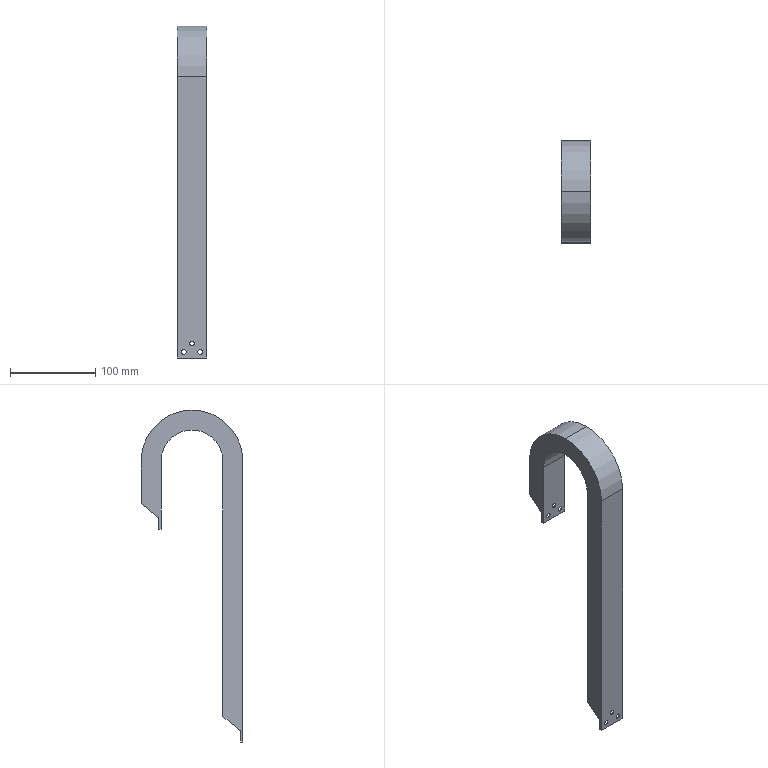Part | SolidWorks | features 3DProfileFeature 2, Boss 2, HoleWzd 2, Rib 2, MirrorPattern 1, Sweep 1 | 1 solid | 56 faces | box 35 x 119.5 x 389.75 mm | volume 194419 mm3 | plane 24 | cylinder 20 | cone 12 | commonest cylinder face diameters 5.5 x12 72.5 x2 78 x2 114 x2 119.5 x2